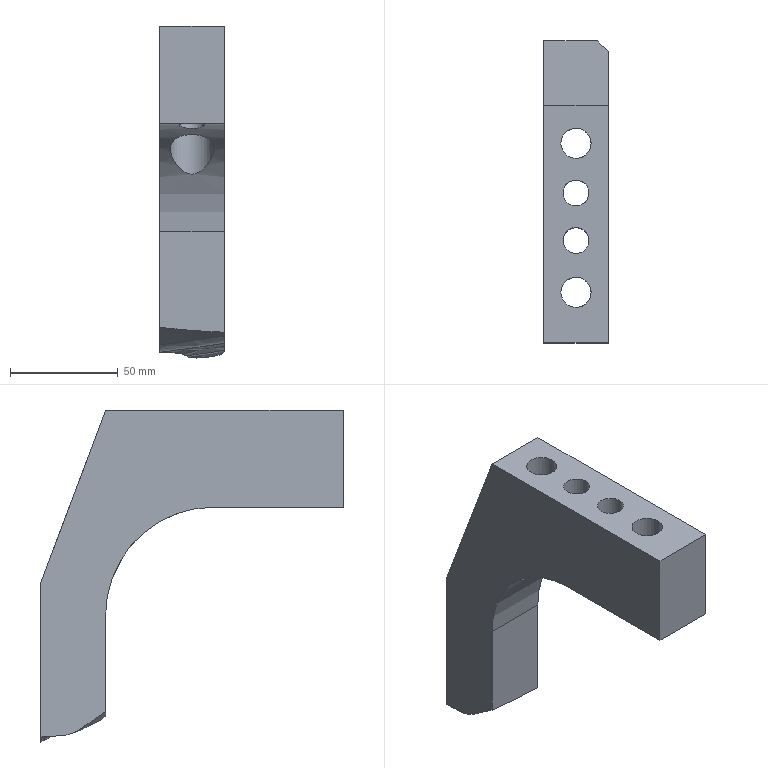Part | NX | features solid 2 | 1 solid | 24 faces | box 30.003 x 140.006 x 153.73 mm | volume 225991 mm3 | plane 11 | cylinder 7 | spline 6 | commonest cylinder face diameters 12 x2 14 x2 20 x2 100 x1
STEP:
#1=CARTESIAN_POINT('',(595.389,275.,-50.88));
#2=VERTEX_POINT('',#1);
#3=CARTESIAN_POINT('',(595.389,274.602,-50.209));
#4=VERTEX_POINT('',#3);
#5=CARTESIAN_POINT('',(595.389,275.,-50.88));
#6=CARTESIAN_POINT('',(595.389,274.842,-50.675));
#7=CARTESIAN_POINT('',(595.389,274.707,-50.449));
#8=CARTESIAN_POINT('',(595.389,274.602,-50.209));
#9=B_SPLINE_CURVE_WITH_KNOTS('',3,(#5,#6,#7,#8),.UNSPECIFIED.,.F.,.F.,(4,4),(0.002934,0.003708),.UNSPECIFIED.);
#10=EDGE_CURVE('',#2,#4,#9,.T.);
#11=ORIENTED_EDGE('',*,*,#10,.F.);
#12=CARTESIAN_POINT('',(595.389,275.,33.333));
#13=VERTEX_POINT('',#12);
#14=CARTESIAN_POINT('',(595.389,275.,20.));
#15=DIRECTION('',(0.,0.,1.));
#16=VECTOR('',#15,1000.);
#17=LINE('',#14,#16);
#18=EDGE_CURVE('',#2,#13,#17,.T.);
#19=ORIENTED_EDGE('',*,*,#18,.T.);
#20=CARTESIAN_POINT('',(595.389,250.,100.));
#21=VERTEX_POINT('',#20);
#22=CARTESIAN_POINT('',(595.389,339.439,-138.505));
#23=DIRECTION('',(0.,0.3511,-0.9363));
#24=VECTOR('',#23,1000.);
#25=LINE('',#22,#24);
#26=EDGE_CURVE('',#13,#21,#25,.F.);
#27=ORIENTED_EDGE('',*,*,#26,.T.);
#28=CARTESIAN_POINT('',(595.389,140.,100.));
#29=VERTEX_POINT('',#28);
#30=CARTESIAN_POINT('',(595.389,175.452,100.));
#31=DIRECTION('',(0.,1.,0.));
#32=VECTOR('',#31,1000.);
#33=LINE('',#30,#32);
#34=EDGE_CURVE('',#29,#21,#33,.T.);
#35=ORIENTED_EDGE('',*,*,#34,.F.);
#36=CARTESIAN_POINT('',(595.389,140.,55.));
#37=VERTEX_POINT('',#36);
#38=CARTESIAN_POINT('',(595.389,140.,-200.));
#39=DIRECTION('',(0.,0.,1.));
#40=VECTOR('',#39,1000.);
#41=LINE('',#38,#40);
#42=EDGE_CURVE('',#37,#29,#41,.T.);
#43=ORIENTED_EDGE('',*,*,#42,.F.);
#44=CARTESIAN_POINT('',(595.389,200.,55.));
#45=VERTEX_POINT('',#44);
#46=CARTESIAN_POINT('',(595.389,175.452,55.));
#47=DIRECTION('',(0.,1.,0.));
#48=VECTOR('',#47,1000.);
#49=LINE('',#46,#48);
#50=EDGE_CURVE('',#37,#45,#49,.T.);
#51=ORIENTED_EDGE('',*,*,#50,.T.);
#52=CARTESIAN_POINT('',(595.389,250.,5.));
#53=VERTEX_POINT('',#52);
#54=CARTESIAN_POINT('',(595.389,200.,5.));
#55=DIRECTION('',(1.,0.,0.));
#56=DIRECTION('',(0.,1.,0.));
#57=AXIS2_PLACEMENT_3D('',#54,#55,#56);
#58=CIRCLE('',#57,50.);
#59=EDGE_CURVE('',#45,#53,#58,.F.);
#60=ORIENTED_EDGE('',*,*,#59,.T.);
#61=CARTESIAN_POINT('',(595.389,250.,-41.794));
#62=VERTEX_POINT('',#61);
#63=CARTESIAN_POINT('',(595.389,250.,-200.));
#64=DIRECTION('',(0.,0.,1.));
#65=VECTOR('',#64,1000.);
#66=LINE('',#63,#65);
#67=EDGE_CURVE('',#62,#53,#66,.T.);
#68=ORIENTED_EDGE('',*,*,#67,.F.);
#69=CARTESIAN_POINT('',(595.389,252.457,-43.548));
#70=VERTEX_POINT('',#69);
#71=CARTESIAN_POINT('',(595.389,252.459,-43.549));
#72=CARTESIAN_POINT('',(595.389,251.639,-42.964));
#73=CARTESIAN_POINT('',(595.389,250.82,-42.379));
#74=CARTESIAN_POINT('',(595.389,250.,-41.794));
#75=B_SPLINE_CURVE_WITH_KNOTS('',3,(#71,#72,#73,#74),.UNSPECIFIED.,.F.,.F.,(4,4),(0.0001783,0.003199),.UNSPECIFIED.);
#76=EDGE_CURVE('',#70,#62,#75,.T.);
#77=ORIENTED_EDGE('',*,*,#76,.F.);
#78=CARTESIAN_POINT('',(595.389,262.065,-46.788));
#79=VERTEX_POINT('',#78);
#80=CARTESIAN_POINT('',(595.389,262.069,-46.789));
#81=CARTESIAN_POINT('',(595.389,258.623,-46.693));
#82=CARTESIAN_POINT('',(595.389,255.262,-45.551));
#83=CARTESIAN_POINT('',(595.389,252.457,-43.548));
#84=B_SPLINE_CURVE_WITH_KNOTS('',3,(#80,#81,#82,#83),.UNSPECIFIED.,.F.,.F.,(4,4),(0.,0.01023),.UNSPECIFIED.);
#85=EDGE_CURVE('',#79,#70,#84,.T.);
#86=ORIENTED_EDGE('',*,*,#85,.F.);
#87=CARTESIAN_POINT('',(595.389,269.735,-46.971));
#88=VERTEX_POINT('',#87);
#89=CARTESIAN_POINT('',(595.389,262.064,-46.788));
#90=CARTESIAN_POINT('',(595.389,264.616,-46.859));
#91=CARTESIAN_POINT('',(595.389,267.169,-46.92));
#92=CARTESIAN_POINT('',(595.389,269.721,-46.971));
#93=B_SPLINE_CURVE_WITH_KNOTS('',3,(#89,#90,#91,#92),.UNSPECIFIED.,.F.,.F.,(4,4),(0.0001094,0.007768),.UNSPECIFIED.);
#94=EDGE_CURVE('',#79,#88,#93,.T.);
#95=ORIENTED_EDGE('',*,*,#94,.T.);
#96=CARTESIAN_POINT('',(595.389,274.603,-50.211));
#97=CARTESIAN_POINT('',(595.389,273.774,-48.31));
#98=CARTESIAN_POINT('',(595.389,271.814,-47.013));
#99=CARTESIAN_POINT('',(595.389,269.74,-46.971));
#100=B_SPLINE_CURVE_WITH_KNOTS('',3,(#96,#97,#98,#99),.UNSPECIFIED.,.F.,.F.,(4,4),(0.,0.006132),.UNSPECIFIED.);
#101=EDGE_CURVE('',#4,#88,#100,.T.);
#102=ORIENTED_EDGE('',*,*,#101,.F.);
#103=EDGE_LOOP('',(#11,#19,#27,#35,#43,#51,#60,#68,#77,#86,#95,#102));
#104=FACE_BOUND('',#103,.T.);
#105=CARTESIAN_POINT('',(595.389,175.452,-200.));
#106=DIRECTION('',(1.,0.,0.));
#107=DIRECTION('',(0.,0.,-1.));
#108=AXIS2_PLACEMENT_3D('',#105,#106,#107);
#109=PLANE('',#108);
#110=ADVANCED_FACE('',(#104),#109,.T.);
#111=CARTESIAN_POINT('',(565.389,140.,100.));
#112=VERTEX_POINT('',#111);
#113=CARTESIAN_POINT('',(565.389,250.,100.));
#114=VERTEX_POINT('',#113);
#115=CARTESIAN_POINT('',(565.389,175.452,100.));
#116=DIRECTION('',(0.,1.,0.));
#117=VECTOR('',#116,1000.);
#118=LINE('',#115,#117);
#119=EDGE_CURVE('',#112,#114,#118,.T.);
#120=ORIENTED_EDGE('',*,*,#119,.T.);
#121=CARTESIAN_POINT('',(565.389,280.,20.));
#122=VERTEX_POINT('',#121);
#123=CARTESIAN_POINT('',(565.389,250.,100.));
#124=DIRECTION('',(0.,-0.3511,0.9363));
#125=VECTOR('',#124,1000.);
#126=LINE('',#123,#125);
#127=EDGE_CURVE('',#114,#122,#126,.F.);
#128=ORIENTED_EDGE('',*,*,#127,.T.);
#129=CARTESIAN_POINT('',(565.389,280.,-51.188));
#130=VERTEX_POINT('',#129);
#131=CARTESIAN_POINT('',(565.389,280.,-200.));
#132=DIRECTION('',(0.,0.,-1.));
#133=VECTOR('',#132,1000.);
#134=LINE('',#131,#133);
#135=EDGE_CURVE('',#122,#130,#134,.T.);
#136=ORIENTED_EDGE('',*,*,#135,.T.);
#137=CARTESIAN_POINT('',(565.389,279.203,-51.114));
#138=VERTEX_POINT('',#137);
#139=CARTESIAN_POINT('',(565.389,280.,-51.188));
#140=CARTESIAN_POINT('',(565.389,279.737,-51.145));
#141=CARTESIAN_POINT('',(565.389,279.473,-51.12));
#142=CARTESIAN_POINT('',(565.389,279.206,-51.114));
#143=B_SPLINE_CURVE_WITH_KNOTS('',3,(#139,#140,#141,#142),.UNSPECIFIED.,.F.,.F.,(4,4),(0.,0.0007971),.UNSPECIFIED.);
#144=EDGE_CURVE('',#130,#138,#143,.T.);
#145=ORIENTED_EDGE('',*,*,#144,.T.);
#146=CARTESIAN_POINT('',(565.389,271.356,-50.91));
#147=VERTEX_POINT('',#146);
#148=CARTESIAN_POINT('',(565.389,271.354,-50.91));
#149=CARTESIAN_POINT('',(565.389,273.966,-50.989));
#150=CARTESIAN_POINT('',(565.389,276.579,-51.057));
#151=CARTESIAN_POINT('',(565.389,279.191,-51.114));
#152=B_SPLINE_CURVE_WITH_KNOTS('',3,(#148,#149,#150,#151),.UNSPECIFIED.,.F.,.F.,(4,4),(0.00007643,0.007916),.UNSPECIFIED.);
#153=EDGE_CURVE('',#147,#138,#152,.T.);
#154=ORIENTED_EDGE('',*,*,#153,.F.);
#155=CARTESIAN_POINT('',(565.389,261.52,-47.642));
#156=VERTEX_POINT('',#155);
#157=CARTESIAN_POINT('',(565.389,271.357,-50.91));
#158=CARTESIAN_POINT('',(565.389,267.84,-50.803));
#159=CARTESIAN_POINT('',(565.389,264.401,-49.662));
#160=CARTESIAN_POINT('',(565.389,261.519,-47.641));
#161=B_SPLINE_CURVE_WITH_KNOTS('',3,(#157,#158,#159,#160),.UNSPECIFIED.,.F.,.F.,(4,4),(0.,0.01045),.UNSPECIFIED.);
#162=EDGE_CURVE('',#147,#156,#161,.T.);
#163=ORIENTED_EDGE('',*,*,#162,.T.);
#164=CARTESIAN_POINT('',(565.389,250.,-39.567));
#165=VERTEX_POINT('',#164);
#166=CARTESIAN_POINT('',(565.389,261.522,-47.643));
#167=CARTESIAN_POINT('',(565.389,257.681,-44.95));
#168=CARTESIAN_POINT('',(565.389,253.841,-42.258));
#169=CARTESIAN_POINT('',(565.389,250.,-39.567));
#170=B_SPLINE_CURVE_WITH_KNOTS('',3,(#166,#167,#168,#169),.UNSPECIFIED.,.F.,.F.,(4,4),(0.0001843,0.01425),.UNSPECIFIED.);
#171=EDGE_CURVE('',#156,#165,#170,.T.);
#172=ORIENTED_EDGE('',*,*,#171,.T.);
#173=CARTESIAN_POINT('',(565.389,250.,5.));
#174=VERTEX_POINT('',#173);
#175=CARTESIAN_POINT('',(565.389,250.,-200.));
#176=DIRECTION('',(0.,0.,1.));
#177=VECTOR('',#176,1000.);
#178=LINE('',#175,#177);
#179=EDGE_CURVE('',#165,#174,#178,.T.);
#180=ORIENTED_EDGE('',*,*,#179,.T.);
#181=CARTESIAN_POINT('',(565.389,200.,55.));
#182=VERTEX_POINT('',#181);
#183=CARTESIAN_POINT('',(565.389,200.,5.));
#184=DIRECTION('',(1.,0.,0.));
#185=DIRECTION('',(0.,1.,0.));
#186=AXIS2_PLACEMENT_3D('',#183,#184,#185);
#187=CIRCLE('',#186,50.);
#188=EDGE_CURVE('',#174,#182,#187,.T.);
#189=ORIENTED_EDGE('',*,*,#188,.T.);
#190=CARTESIAN_POINT('',(565.389,140.,55.));
#191=VERTEX_POINT('',#190);
#192=CARTESIAN_POINT('',(565.389,255.452,55.));
#193=DIRECTION('',(0.,1.,0.));
#194=VECTOR('',#193,1000.);
#195=LINE('',#192,#194);
#196=EDGE_CURVE('',#182,#191,#195,.F.);
#197=ORIENTED_EDGE('',*,*,#196,.T.);
#198=CARTESIAN_POINT('',(565.389,140.,-200.));
#199=DIRECTION('',(0.,0.,1.));
#200=VECTOR('',#199,1000.);
#201=LINE('',#198,#200);
#202=EDGE_CURVE('',#191,#112,#201,.T.);
#203=ORIENTED_EDGE('',*,*,#202,.T.);
#204=EDGE_LOOP('',(#120,#128,#136,#145,#154,#163,#172,#180,#189,#197,#203));
#205=FACE_BOUND('',#204,.T.);
#206=CARTESIAN_POINT('',(565.389,175.452,-200.));
#207=DIRECTION('',(1.,0.,0.));
#208=DIRECTION('',(0.,0.,-1.));
#209=AXIS2_PLACEMENT_3D('',#206,#207,#208);
#210=PLANE('',#209);
#211=ADVANCED_FACE('',(#205),#210,.F.);
#212=CARTESIAN_POINT('',(575.439,227.503,100.));
#213=VERTEX_POINT('',#212);
#214=CARTESIAN_POINT('',(580.389,232.452,100.));
#215=DIRECTION('',(0.,0.,-1.));
#216=DIRECTION('',(-0.7071,-0.7071,0.));
#217=AXIS2_PLACEMENT_3D('',#214,#215,#216);
#218=CIRCLE('',#217,7.);
#219=EDGE_CURVE('',#213,#213,#218,.T.);
#220=ORIENTED_EDGE('',*,*,#219,.T.);
#221=EDGE_LOOP('',(#220));
#222=FACE_BOUND('',#221,.T.);
#223=CARTESIAN_POINT('',(575.439,158.503,100.));
#224=VERTEX_POINT('',#223);
#225=CARTESIAN_POINT('',(580.389,163.452,100.));
#226=DIRECTION('',(0.,0.,-1.));
#227=DIRECTION('',(-0.7071,-0.7071,0.));
#228=AXIS2_PLACEMENT_3D('',#225,#226,#227);
#229=CIRCLE('',#228,7.);
#230=EDGE_CURVE('',#224,#224,#229,.T.);
#231=ORIENTED_EDGE('',*,*,#230,.T.);
#232=EDGE_LOOP('',(#231));
#233=FACE_BOUND('',#232,.T.);
#234=CARTESIAN_POINT('',(576.146,205.21,100.));
#235=VERTEX_POINT('',#234);
#236=CARTESIAN_POINT('',(580.389,209.452,100.));
#237=DIRECTION('',(0.,0.,-1.));
#238=DIRECTION('',(-0.7071,-0.7071,0.));
#239=AXIS2_PLACEMENT_3D('',#236,#237,#238);
#240=CIRCLE('',#239,6.);
#241=EDGE_CURVE('',#235,#235,#240,.T.);
#242=ORIENTED_EDGE('',*,*,#241,.T.);
#243=EDGE_LOOP('',(#242));
#244=FACE_BOUND('',#243,.T.);
#245=CARTESIAN_POINT('',(576.146,183.21,100.));
#246=VERTEX_POINT('',#245);
#247=CARTESIAN_POINT('',(580.389,187.452,100.));
#248=DIRECTION('',(0.,0.,-1.));
#249=DIRECTION('',(-0.7071,-0.7071,0.));
#250=AXIS2_PLACEMENT_3D('',#247,#248,#249);
#251=CIRCLE('',#250,6.);
#252=EDGE_CURVE('',#246,#246,#251,.T.);
#253=ORIENTED_EDGE('',*,*,#252,.T.);
#254=EDGE_LOOP('',(#253));
#255=FACE_BOUND('',#254,.T.);
#256=ORIENTED_EDGE('',*,*,#34,.T.);
#257=CARTESIAN_POINT('',(520.389,250.,100.));
#258=DIRECTION('',(-1.,0.,0.));
#259=VECTOR('',#258,1000.);
#260=LINE('',#257,#259);
#261=EDGE_CURVE('',#21,#114,#260,.T.);
#262=ORIENTED_EDGE('',*,*,#261,.T.);
#263=ORIENTED_EDGE('',*,*,#119,.F.);
#264=CARTESIAN_POINT('',(635.389,140.,100.));
#265=DIRECTION('',(-1.,0.,0.));
#266=VECTOR('',#265,1000.);
#267=LINE('',#264,#266);
#268=EDGE_CURVE('',#29,#112,#267,.T.);
#269=ORIENTED_EDGE('',*,*,#268,.F.);
#270=EDGE_LOOP('',(#256,#262,#263,#269));
#271=FACE_BOUND('',#270,.T.);
#272=CARTESIAN_POINT('',(520.389,175.452,100.));
#273=DIRECTION('',(0.,0.,-1.));
#274=DIRECTION('',(-1.,0.,0.));
#275=AXIS2_PLACEMENT_3D('',#272,#273,#274);
#276=PLANE('',#275);
#277=ADVANCED_FACE('',(#222,#233,#244,#255,#271),#276,.F.);
#278=CARTESIAN_POINT('',(590.389,163.452,55.));
#279=VERTEX_POINT('',#278);
#280=CARTESIAN_POINT('',(580.389,163.452,55.));
#281=DIRECTION('',(0.,0.,1.));
#282=DIRECTION('',(1.,0.,0.));
#283=AXIS2_PLACEMENT_3D('',#280,#281,#282);
#284=CIRCLE('',#283,10.);
#285=EDGE_CURVE('',#279,#279,#284,.F.);
#286=ORIENTED_EDGE('',*,*,#285,.F.);
#287=EDGE_LOOP('',(#286));
#288=FACE_BOUND('',#287,.T.);
#289=CARTESIAN_POINT('',(574.389,187.452,55.));
#290=VERTEX_POINT('',#289);
#291=CARTESIAN_POINT('',(580.389,187.452,55.));
#292=DIRECTION('',(0.,0.,-1.));
#293=DIRECTION('',(-1.,0.,0.));
#294=AXIS2_PLACEMENT_3D('',#291,#292,#293);
#295=CIRCLE('',#294,6.);
#296=EDGE_CURVE('',#290,#290,#295,.T.);
#297=ORIENTED_EDGE('',*,*,#296,.F.);
#298=EDGE_LOOP('',(#297));
#299=FACE_BOUND('',#298,.T.);
#300=ORIENTED_EDGE('',*,*,#196,.F.);
#301=CARTESIAN_POINT('',(595.389,200.,55.));
#302=DIRECTION('',(-1.,0.,0.));
#303=VECTOR('',#302,1000.);
#304=LINE('',#301,#303);
#305=EDGE_CURVE('',#182,#45,#304,.F.);
#306=ORIENTED_EDGE('',*,*,#305,.T.);
#307=ORIENTED_EDGE('',*,*,#50,.F.);
#308=CARTESIAN_POINT('',(595.389,140.,55.));
#309=DIRECTION('',(-1.,0.,0.));
#310=VECTOR('',#309,1000.);
#311=LINE('',#308,#310);
#312=EDGE_CURVE('',#37,#191,#311,.T.);
#313=ORIENTED_EDGE('',*,*,#312,.T.);
#314=EDGE_LOOP('',(#300,#306,#307,#313));
#315=FACE_BOUND('',#314,.T.);
#316=CARTESIAN_POINT('',(595.389,255.452,55.));
#317=DIRECTION('',(0.,0.,1.));
#318=DIRECTION('',(1.,0.,0.));
#319=AXIS2_PLACEMENT_3D('',#316,#317,#318);
#320=PLANE('',#319);
#321=ADVANCED_FACE('',(#288,#299,#315),#320,.F.);
#322=ORIENTED_EDGE('',*,*,#202,.F.);
#323=ORIENTED_EDGE('',*,*,#312,.F.);
#324=ORIENTED_EDGE('',*,*,#42,.T.);
#325=ORIENTED_EDGE('',*,*,#268,.T.);
#326=EDGE_LOOP('',(#322,#323,#324,#325));
#327=FACE_BOUND('',#326,.T.);
#328=CARTESIAN_POINT('',(635.389,140.,75.));
#329=DIRECTION('',(0.,1.,0.));
#330=DIRECTION('',(0.,0.,1.));
#331=AXIS2_PLACEMENT_3D('',#328,#329,#330);
#332=PLANE('',#331);
#333=ADVANCED_FACE('',(#327),#332,.F.);
#334=CARTESIAN_POINT('',(587.389,232.452,75.));
#335=VERTEX_POINT('',#334);
#336=CARTESIAN_POINT('',(580.389,232.452,75.));
#337=DIRECTION('',(0.,0.,1.));
#338=DIRECTION('',(1.,0.,0.));
#339=AXIS2_PLACEMENT_3D('',#336,#337,#338);
#340=CIRCLE('',#339,7.);
#341=EDGE_CURVE('',#335,#335,#340,.T.);
#342=ORIENTED_EDGE('',*,*,#341,.F.);
#343=EDGE_LOOP('',(#342));
#344=FACE_BOUND('',#343,.T.);
#345=ORIENTED_EDGE('',*,*,#219,.F.);
#346=EDGE_LOOP('',(#345));
#347=FACE_BOUND('',#346,.T.);
#348=CARTESIAN_POINT('',(580.389,232.452,75.));
#349=DIRECTION('',(0.,0.,1.));
#350=DIRECTION('',(-1.,0.,0.));
#351=AXIS2_PLACEMENT_3D('',#348,#349,#350);
#352=CYLINDRICAL_SURFACE('',#351,7.);
#353=ADVANCED_FACE('',(#344,#347),#352,.F.);
#354=ORIENTED_EDGE('',*,*,#341,.T.);
#355=EDGE_LOOP('',(#354));
#356=FACE_BOUND('',#355,.T.);
#357=CARTESIAN_POINT('',(590.389,232.452,75.));
#358=VERTEX_POINT('',#357);
#359=CARTESIAN_POINT('',(580.389,232.452,75.));
#360=DIRECTION('',(0.,0.,-1.));
#361=DIRECTION('',(1.,0.,0.));
#362=AXIS2_PLACEMENT_3D('',#359,#360,#361);
#363=CIRCLE('',#362,10.);
#364=EDGE_CURVE('',#358,#358,#363,.T.);
#365=ORIENTED_EDGE('',*,*,#364,.T.);
#366=EDGE_LOOP('',(#365));
#367=FACE_BOUND('',#366,.T.);
#368=CARTESIAN_POINT('',(580.389,232.452,75.));
#369=DIRECTION('',(0.,0.,1.));
#370=DIRECTION('',(-1.,0.,0.));
#371=AXIS2_PLACEMENT_3D('',#368,#369,#370);
#372=PLANE('',#371);
#373=ADVANCED_FACE('',(#356,#367),#372,.F.);
#374=CARTESIAN_POINT('',(571.633,227.622,46.677));
#375=VERTEX_POINT('',#374);
#376=CARTESIAN_POINT('',(574.156,224.201,48.791));
#377=CARTESIAN_POINT('',(571.35,227.566,46.791));
#378=CARTESIAN_POINT('',(570.238,231.271,44.109));
#379=CARTESIAN_POINT('',(570.471,234.796,41.005));
#380=CARTESIAN_POINT('',(571.78,237.887,37.725));
#381=CARTESIAN_POINT('',(573.658,240.016,35.024));
#382=CARTESIAN_POINT('',(575.727,241.369,33.098));
#383=CARTESIAN_POINT('',(577.614,242.141,31.917));
#384=CARTESIAN_POINT('',(579.896,242.535,31.281));
#385=CARTESIAN_POINT('',(582.271,242.362,31.564));
#386=CARTESIAN_POINT('',(584.326,241.718,32.574));
#387=CARTESIAN_POINT('',(586.565,240.483,34.386));
#388=CARTESIAN_POINT('',(588.607,238.463,37.042));
#389=CARTESIAN_POINT('',(590.116,235.478,40.331));
#390=CARTESIAN_POINT('',(590.592,232.039,43.482));
#391=CARTESIAN_POINT('',(589.784,228.323,46.286));
#392=CARTESIAN_POINT('',(587.347,224.824,48.449));
#393=CARTESIAN_POINT('',(583.305,222.502,49.656));
#394=CARTESIAN_POINT('',(578.48,222.255,49.774));
#395=CARTESIAN_POINT('',(574.156,224.201,48.791));
#396=CARTESIAN_POINT('',(571.35,227.566,46.791));
#397=CARTESIAN_POINT('',(570.238,231.271,44.109));
#398=B_SPLINE_CURVE_WITH_KNOTS('',3,(#376,#377,#378,#379,#380,#381,#382,#383,#384,#385,#386,#387,#388,#389,#390,#391,#392,#393,#394,#395,#396,#397),.UNSPECIFIED.,.T.,.F.,(1,1,1,1,1,1,1,1,1,1,1,1,1,1,1,1,1,1,1,1,1,1,1,1,1,1),(-0.01388,-0.009257,-0.004628,0.,0.004628,0.009257,0.01388,0.01851,0.02083,0.02314,0.02546,0.02777,0.03008,0.0324,0.03703,0.04165,0.04628,0.05091,0.05554,0.06017,0.0648,0.06942,0.07405,0.07868,0.08331,0.08794),.UNSPECIFIED.);
#399=EDGE_CURVE('',#375,#375,#398,.T.);
#400=ORIENTED_EDGE('',*,*,#399,.T.);
#401=EDGE_LOOP('',(#400));
#402=FACE_BOUND('',#401,.T.);
#403=ORIENTED_EDGE('',*,*,#364,.F.);
#404=EDGE_LOOP('',(#403));
#405=FACE_BOUND('',#404,.T.);
#406=CARTESIAN_POINT('',(580.389,232.452,75.));
#407=DIRECTION('',(0.,0.,-1.));
#408=DIRECTION('',(1.,0.,0.));
#409=AXIS2_PLACEMENT_3D('',#406,#407,#408);
#410=CYLINDRICAL_SURFACE('',#409,10.);
#411=ADVANCED_FACE('',(#402,#405),#410,.F.);
#412=CARTESIAN_POINT('',(587.389,163.452,75.));
#413=VERTEX_POINT('',#412);
#414=CARTESIAN_POINT('',(580.389,163.452,75.));
#415=DIRECTION('',(0.,0.,1.));
#416=DIRECTION('',(1.,0.,0.));
#417=AXIS2_PLACEMENT_3D('',#414,#415,#416);
#418=CIRCLE('',#417,7.);
#419=EDGE_CURVE('',#413,#413,#418,.T.);
#420=ORIENTED_EDGE('',*,*,#419,.F.);
#421=EDGE_LOOP('',(#420));
#422=FACE_BOUND('',#421,.T.);
#423=ORIENTED_EDGE('',*,*,#230,.F.);
#424=EDGE_LOOP('',(#423));
#425=FACE_BOUND('',#424,.T.);
#426=CARTESIAN_POINT('',(580.389,163.452,75.));
#427=DIRECTION('',(0.,0.,1.));
#428=DIRECTION('',(-1.,0.,0.));
#429=AXIS2_PLACEMENT_3D('',#426,#427,#428);
#430=CYLINDRICAL_SURFACE('',#429,7.);
#431=ADVANCED_FACE('',(#422,#425),#430,.F.);
#432=ORIENTED_EDGE('',*,*,#285,.T.);
#433=EDGE_LOOP('',(#432));
#434=FACE_BOUND('',#433,.T.);
#435=CARTESIAN_POINT('',(590.389,163.452,75.));
#436=VERTEX_POINT('',#435);
#437=CARTESIAN_POINT('',(580.389,163.452,75.));
#438=DIRECTION('',(0.,0.,-1.));
#439=DIRECTION('',(1.,0.,0.));
#440=AXIS2_PLACEMENT_3D('',#437,#438,#439);
#441=CIRCLE('',#440,10.);
#442=EDGE_CURVE('',#436,#436,#441,.T.);
#443=ORIENTED_EDGE('',*,*,#442,.F.);
#444=EDGE_LOOP('',(#443));
#445=FACE_BOUND('',#444,.T.);
#446=CARTESIAN_POINT('',(580.389,163.452,75.));
#447=DIRECTION('',(0.,0.,-1.));
#448=DIRECTION('',(1.,0.,0.));
#449=AXIS2_PLACEMENT_3D('',#446,#447,#448);
#450=CYLINDRICAL_SURFACE('',#449,10.);
#451=ADVANCED_FACE('',(#434,#445),#450,.F.);
#452=ORIENTED_EDGE('',*,*,#419,.T.);
#453=EDGE_LOOP('',(#452));
#454=FACE_BOUND('',#453,.T.);
#455=ORIENTED_EDGE('',*,*,#442,.T.);
#456=EDGE_LOOP('',(#455));
#457=FACE_BOUND('',#456,.T.);
#458=CARTESIAN_POINT('',(580.389,163.452,75.));
#459=DIRECTION('',(0.,0.,1.));
#460=DIRECTION('',(-1.,0.,0.));
#461=AXIS2_PLACEMENT_3D('',#458,#459,#460);
#462=PLANE('',#461);
#463=ADVANCED_FACE('',(#454,#457),#462,.F.);
#464=ORIENTED_EDGE('',*,*,#241,.F.);
#465=EDGE_LOOP('',(#464));
#466=FACE_BOUND('',#465,.T.);
#467=CARTESIAN_POINT('',(586.387,209.288,54.13));
#468=VERTEX_POINT('',#467);
#469=CARTESIAN_POINT('',(585.262,213.959,53.061));
#470=CARTESIAN_POINT('',(587.022,209.288,54.223));
#471=CARTESIAN_POINT('',(584.969,204.616,54.826));
#472=CARTESIAN_POINT('',(580.154,202.791,54.914));
#473=CARTESIAN_POINT('',(575.472,204.957,54.8));
#474=CARTESIAN_POINT('',(573.765,209.756,54.132));
#475=CARTESIAN_POINT('',(575.834,214.279,52.959));
#476=CARTESIAN_POINT('',(580.62,216.114,52.325));
#477=CARTESIAN_POINT('',(585.262,213.959,53.061));
#478=CARTESIAN_POINT('',(587.022,209.288,54.223));
#479=CARTESIAN_POINT('',(584.969,204.616,54.826));
#480=B_SPLINE_CURVE_WITH_KNOTS('',3,(#469,#470,#471,#472,#473,#474,#475,#476,#477,#478,#479),.UNSPECIFIED.,.T.,.F.,(1,1,1,1,1,1,1,1,1,1,1,1,1,1,1),(-0.01421,-0.009475,-0.004737,0.,0.004737,0.009475,0.01421,0.01895,0.02369,0.02842,0.03316,0.0379,0.04264,0.04737,0.05211),.UNSPECIFIED.);
#481=EDGE_CURVE('',#468,#468,#480,.T.);
#482=ORIENTED_EDGE('',*,*,#481,.T.);
#483=EDGE_LOOP('',(#482));
#484=FACE_BOUND('',#483,.T.);
#485=CARTESIAN_POINT('',(580.389,209.452,105.));
#486=DIRECTION('',(0.,0.,-1.));
#487=DIRECTION('',(-1.,0.,0.));
#488=AXIS2_PLACEMENT_3D('',#485,#486,#487);
#489=CYLINDRICAL_SURFACE('',#488,6.);
#490=ADVANCED_FACE('',(#466,#484),#489,.F.);
#491=ORIENTED_EDGE('',*,*,#252,.F.);
#492=EDGE_LOOP('',(#491));
#493=FACE_BOUND('',#492,.T.);
#494=ORIENTED_EDGE('',*,*,#296,.T.);
#495=EDGE_LOOP('',(#494));
#496=FACE_BOUND('',#495,.T.);
#497=CARTESIAN_POINT('',(580.389,187.452,105.));
#498=DIRECTION('',(0.,0.,-1.));
#499=DIRECTION('',(-1.,0.,0.));
#500=AXIS2_PLACEMENT_3D('',#497,#498,#499);
#501=CYLINDRICAL_SURFACE('',#500,6.);
#502=ADVANCED_FACE('',(#493,#496),#501,.F.);
#503=ORIENTED_EDGE('',*,*,#67,.T.);
#504=CARTESIAN_POINT('',(565.389,250.,5.));
#505=DIRECTION('',(-1.,0.,0.));
#506=VECTOR('',#505,1000.);
#507=LINE('',#504,#506);
#508=EDGE_CURVE('',#53,#174,#507,.T.);
#509=ORIENTED_EDGE('',*,*,#508,.T.);
#510=ORIENTED_EDGE('',*,*,#179,.F.);
#511=CARTESIAN_POINT('',(565.389,250.,-39.567));
#512=CARTESIAN_POINT('',(575.36,250.,-40.699));
#513=CARTESIAN_POINT('',(585.358,250.,-41.464));
#514=CARTESIAN_POINT('',(595.389,250.,-41.794));
#515=B_SPLINE_CURVE_WITH_KNOTS('',3,(#511,#512,#513,#514),.UNSPECIFIED.,.F.,.F.,(4,4),(0.,0.03008),.UNSPECIFIED.);
#516=EDGE_CURVE('',#165,#62,#515,.T.);
#517=ORIENTED_EDGE('',*,*,#516,.T.);
#518=EDGE_LOOP('',(#503,#509,#510,#517));
#519=FACE_BOUND('',#518,.T.);
#520=CARTESIAN_POINT('',(580.389,250.,4.472));
#521=DIRECTION('',(0.,1.,0.));
#522=DIRECTION('',(-1.,0.,0.));
#523=AXIS2_PLACEMENT_3D('',#520,#521,#522);
#524=PLANE('',#523);
#525=ADVANCED_FACE('',(#519),#524,.F.);
#526=CARTESIAN_POINT('',(590.389,280.,20.));
#527=VERTEX_POINT('',#526);
#528=CARTESIAN_POINT('',(580.389,280.,20.));
#529=DIRECTION('',(1.,0.,0.));
#530=VECTOR('',#529,1000.);
#531=LINE('',#528,#530);
#532=EDGE_CURVE('',#122,#527,#531,.T.);
#533=ORIENTED_EDGE('',*,*,#532,.T.);
#534=CARTESIAN_POINT('',(590.389,280.,-52.923));
#535=VERTEX_POINT('',#534);
#536=CARTESIAN_POINT('',(590.389,280.,-52.18));
#537=DIRECTION('',(0.,0.,-1.));
#538=VECTOR('',#537,1000.);
#539=LINE('',#536,#538);
#540=EDGE_CURVE('',#527,#535,#539,.T.);
#541=ORIENTED_EDGE('',*,*,#540,.T.);
#542=CARTESIAN_POINT('',(586.939,280.,-53.416));
#543=VERTEX_POINT('',#542);
#544=CARTESIAN_POINT('',(590.389,280.,-52.923));
#545=CARTESIAN_POINT('',(589.232,280.,-53.091));
#546=CARTESIAN_POINT('',(588.074,280.,-53.257));
#547=CARTESIAN_POINT('',(586.917,280.,-53.42));
#548=B_SPLINE_CURVE_WITH_KNOTS('',3,(#544,#545,#546,#547),.UNSPECIFIED.,.F.,.F.,(4,4),(0.005054,0.008561),.UNSPECIFIED.);
#549=EDGE_CURVE('',#535,#543,#548,.T.);
#550=ORIENTED_EDGE('',*,*,#549,.T.);
#551=CARTESIAN_POINT('',(577.508,280.,-52.788));
#552=VERTEX_POINT('',#551);
#553=CARTESIAN_POINT('',(586.96,280.,-53.413));
#554=CARTESIAN_POINT('',(585.374,280.,-53.637));
#555=CARTESIAN_POINT('',(582.969,280.,-53.826));
#556=CARTESIAN_POINT('',(579.782,280.,-53.577));
#557=CARTESIAN_POINT('',(578.2,280.,-53.206));
#558=CARTESIAN_POINT('',(577.509,280.,-52.788));
#559=B_SPLINE_CURVE_WITH_KNOTS('',3,(#553,#554,#555,#556,#557,#558),.UNSPECIFIED.,.F.,.F.,(4,1,1,4),(0.,0.004801,0.007201,0.009601),.UNSPECIFIED.);
#560=EDGE_CURVE('',#543,#552,#559,.T.);
#561=ORIENTED_EDGE('',*,*,#560,.T.);
#562=CARTESIAN_POINT('',(577.51,280.,-52.789));
#563=CARTESIAN_POINT('',(576.618,280.,-52.25));
#564=CARTESIAN_POINT('',(574.631,280.,-51.648));
#565=CARTESIAN_POINT('',(570.552,280.,-51.051));
#566=CARTESIAN_POINT('',(567.449,280.,-51.056));
#567=CARTESIAN_POINT('',(565.389,280.,-51.188));
#568=B_SPLINE_CURVE_WITH_KNOTS('',3,(#562,#563,#564,#565,#566,#567),.UNSPECIFIED.,.F.,.F.,(4,1,1,4),(0.,0.003084,0.006167,0.01233),.UNSPECIFIED.);
#569=EDGE_CURVE('',#552,#130,#568,.T.);
#570=ORIENTED_EDGE('',*,*,#569,.T.);
#571=ORIENTED_EDGE('',*,*,#135,.F.);
#572=EDGE_LOOP('',(#533,#541,#550,#561,#570,#571));
#573=FACE_BOUND('',#572,.T.);
#574=CARTESIAN_POINT('',(580.389,280.,77.5));
#575=DIRECTION('',(0.,-1.,0.));
#576=DIRECTION('',(1.,0.,0.));
#577=AXIS2_PLACEMENT_3D('',#574,#575,#576);
#578=PLANE('',#577);
#579=ADVANCED_FACE('',(#573),#578,.F.);
#580=ORIENTED_EDGE('',*,*,#85,.T.);
#581=CARTESIAN_POINT('',(595.388,252.457,-43.548));
#582=CARTESIAN_POINT('',(585.214,255.127,-45.11));
#583=CARTESIAN_POINT('',(575.214,258.15,-46.449));
#584=CARTESIAN_POINT('',(565.388,261.519,-47.641));
#585=B_SPLINE_CURVE_WITH_KNOTS('',3,(#581,#582,#583,#584),.UNSPECIFIED.,.F.,.F.,(4,4),(0.4564,0.6419),.UNSPECIFIED.);
#586=EDGE_CURVE('',#70,#156,#585,.T.);
#587=ORIENTED_EDGE('',*,*,#586,.T.);
#588=ORIENTED_EDGE('',*,*,#162,.F.);
#589=CARTESIAN_POINT('',(565.389,271.357,-50.91));
#590=CARTESIAN_POINT('',(575.205,267.905,-49.708));
#591=CARTESIAN_POINT('',(585.204,264.807,-48.361));
#592=CARTESIAN_POINT('',(595.389,262.069,-46.788));
#593=B_SPLINE_CURVE_WITH_KNOTS('',3,(#589,#590,#591,#592),.UNSPECIFIED.,.F.,.F.,(4,4),(0.3373,0.5274),.UNSPECIFIED.);
#594=EDGE_CURVE('',#147,#79,#593,.T.);
#595=ORIENTED_EDGE('',*,*,#594,.T.);
#596=EDGE_LOOP('',(#580,#587,#588,#595));
#597=FACE_BOUND('',#596,.T.);
#598=CARTESIAN_POINT('',(595.593,252.403,-43.516));
#599=CARTESIAN_POINT('',(596.178,253.928,-44.625));
#600=CARTESIAN_POINT('',(596.771,255.63,-45.486));
#601=CARTESIAN_POINT('',(597.354,257.461,-46.064));
#602=CARTESIAN_POINT('',(597.908,259.36,-46.34));
#603=CARTESIAN_POINT('',(598.416,261.267,-46.315));
#604=CARTESIAN_POINT('',(589.929,253.887,-44.387));
#605=CARTESIAN_POINT('',(590.527,255.405,-45.499));
#606=CARTESIAN_POINT('',(591.137,257.101,-46.362));
#607=CARTESIAN_POINT('',(591.741,258.925,-46.942));
#608=CARTESIAN_POINT('',(592.319,260.817,-47.219));
#609=CARTESIAN_POINT('',(592.853,262.718,-47.196));
#610=CARTESIAN_POINT('',(584.309,255.461,-45.201));
#611=CARTESIAN_POINT('',(584.92,256.974,-46.315));
#612=CARTESIAN_POINT('',(585.548,258.663,-47.18));
#613=CARTESIAN_POINT('',(586.173,260.479,-47.762));
#614=CARTESIAN_POINT('',(586.774,262.365,-48.041));
#615=CARTESIAN_POINT('',(587.335,264.259,-48.019));
#616=CARTESIAN_POINT('',(578.734,257.127,-45.963));
#617=CARTESIAN_POINT('',(579.359,258.633,-47.079));
#618=CARTESIAN_POINT('',(580.004,260.314,-47.947));
#619=CARTESIAN_POINT('',(580.651,262.123,-48.531));
#620=CARTESIAN_POINT('',(581.277,264.002,-48.811));
#621=CARTESIAN_POINT('',(581.863,265.888,-48.79));
#622=CARTESIAN_POINT('',(571.996,259.266,-46.835));
#623=CARTESIAN_POINT('',(572.639,260.763,-47.955));
#624=CARTESIAN_POINT('',(573.306,262.435,-48.825));
#625=CARTESIAN_POINT('',(573.978,264.235,-49.412));
#626=CARTESIAN_POINT('',(574.634,266.103,-49.694));
#627=CARTESIAN_POINT('',(575.252,267.981,-49.674));
#628=CARTESIAN_POINT('',(565.325,261.538,-47.65));
#629=CARTESIAN_POINT('',(565.985,263.026,-48.772));
#630=CARTESIAN_POINT('',(566.675,264.688,-49.645));
#631=CARTESIAN_POINT('',(567.373,266.478,-50.234));
#632=CARTESIAN_POINT('',(568.058,268.336,-50.518));
#633=CARTESIAN_POINT('',(568.707,270.203,-50.5));
#634=CARTESIAN_POINT('',(564.129,261.95,-47.795));
#635=CARTESIAN_POINT('',(564.793,263.437,-48.917));
#636=CARTESIAN_POINT('',(565.487,265.097,-49.791));
#637=CARTESIAN_POINT('',(566.19,266.885,-50.379));
#638=CARTESIAN_POINT('',(566.88,268.741,-50.664));
#639=CARTESIAN_POINT('',(567.535,270.606,-50.646));
#640=CARTESIAN_POINT('',(562.936,262.367,-47.937));
#641=CARTESIAN_POINT('',(563.603,263.851,-49.06));
#642=CARTESIAN_POINT('',(564.301,265.51,-49.934));
#643=CARTESIAN_POINT('',(565.009,267.296,-50.523));
#644=CARTESIAN_POINT('',(565.703,269.15,-50.809));
#645=CARTESIAN_POINT('',(566.364,271.014,-50.791));
#646=CARTESIAN_POINT('',(561.744,262.788,-48.078));
#647=CARTESIAN_POINT('',(562.414,264.271,-49.202));
#648=CARTESIAN_POINT('',(563.117,265.927,-50.076));
#649=CARTESIAN_POINT('',(563.829,267.711,-50.666));
#650=CARTESIAN_POINT('',(564.53,269.564,-50.951));
#651=CARTESIAN_POINT('',(565.196,271.425,-50.933));
#652=B_SPLINE_SURFACE_WITH_KNOTS('',5,5,((#598,#599,#600,#601,#602,#603),(#604,#605,#606,#607,#608,#609),(#610,#611,#612,#613,#614,#615),(#616,#617,#618,#619,#620,#621),(#622,#623,#624,#625,#626,#627),(#628,#629,#630,#631,#632,#633),(#634,#635,#636,#637,#638,#639),(#640,#641,#642,#643,#644,#645),(#646,#647,#648,#649,#650,#651)),.UNSPECIFIED.,.F.,.F.,.F.,(6,3,6),(6,6),(0.4552,0.6272,0.6648),(0.,1.),.UNSPECIFIED.);
#653=ADVANCED_FACE('',(#597),#652,.T.);
#654=ORIENTED_EDGE('',*,*,#594,.F.);
#655=ORIENTED_EDGE('',*,*,#153,.T.);
#656=CARTESIAN_POINT('',(565.386,279.192,-51.114));
#657=CARTESIAN_POINT('',(575.141,275.691,-49.913));
#658=CARTESIAN_POINT('',(585.138,272.528,-48.561));
#659=CARTESIAN_POINT('',(595.386,269.722,-46.971));
#660=B_SPLINE_CURVE_WITH_KNOTS('',3,(#656,#657,#658,#659),.UNSPECIFIED.,.F.,.F.,(4,4),(0.3631,0.5783),.UNSPECIFIED.);
#661=EDGE_CURVE('',#138,#88,#660,.T.);
#662=ORIENTED_EDGE('',*,*,#661,.T.);
#663=ORIENTED_EDGE('',*,*,#94,.F.);
#664=EDGE_LOOP('',(#654,#655,#662,#663));
#665=FACE_BOUND('',#664,.T.);
#666=CARTESIAN_POINT('',(595.57,261.935,-46.758));
#667=CARTESIAN_POINT('',(596.003,263.763,-46.745));
#668=CARTESIAN_POINT('',(596.436,265.591,-46.726));
#669=CARTESIAN_POINT('',(596.869,267.419,-46.702));
#670=CARTESIAN_POINT('',(597.302,269.247,-46.673));
#671=CARTESIAN_POINT('',(594.342,262.266,-46.948));
#672=CARTESIAN_POINT('',(594.781,264.092,-46.935));
#673=CARTESIAN_POINT('',(595.219,265.919,-46.916));
#674=CARTESIAN_POINT('',(595.658,267.745,-46.892));
#675=CARTESIAN_POINT('',(596.096,269.572,-46.863));
#676=CARTESIAN_POINT('',(593.116,262.601,-47.135));
#677=CARTESIAN_POINT('',(593.561,264.426,-47.122));
#678=CARTESIAN_POINT('',(594.005,266.251,-47.104));
#679=CARTESIAN_POINT('',(594.449,268.076,-47.079));
#680=CARTESIAN_POINT('',(594.893,269.901,-47.05));
#681=CARTESIAN_POINT('',(591.894,262.94,-47.319));
#682=CARTESIAN_POINT('',(592.344,264.763,-47.306));
#683=CARTESIAN_POINT('',(592.794,266.587,-47.288));
#684=CARTESIAN_POINT('',(593.244,268.41,-47.264));
#685=CARTESIAN_POINT('',(593.693,270.234,-47.234));
#686=CARTESIAN_POINT('',(585.233,264.816,-48.311));
#687=CARTESIAN_POINT('',(585.714,266.631,-48.299));
#688=CARTESIAN_POINT('',(586.194,268.446,-48.281));
#689=CARTESIAN_POINT('',(586.674,270.261,-48.257));
#690=CARTESIAN_POINT('',(587.154,272.076,-48.227));
#691=CARTESIAN_POINT('',(578.659,266.815,-49.225));
#692=CARTESIAN_POINT('',(579.17,268.621,-49.213));
#693=CARTESIAN_POINT('',(579.681,270.427,-49.196));
#694=CARTESIAN_POINT('',(580.191,272.233,-49.172));
#695=CARTESIAN_POINT('',(580.701,274.039,-49.143));
#696=CARTESIAN_POINT('',(573.347,268.53,-49.925));
#697=CARTESIAN_POINT('',(573.882,270.328,-49.914));
#698=CARTESIAN_POINT('',(574.417,272.126,-49.898));
#699=CARTESIAN_POINT('',(574.951,273.924,-49.875));
#700=CARTESIAN_POINT('',(575.485,275.722,-49.845));
#701=CARTESIAN_POINT('',(568.091,270.325,-50.586));
#702=CARTESIAN_POINT('',(568.65,272.114,-50.576));
#703=CARTESIAN_POINT('',(569.209,273.904,-50.559));
#704=CARTESIAN_POINT('',(569.768,275.694,-50.537));
#705=CARTESIAN_POINT('',(570.326,277.484,-50.508));
#706=CARTESIAN_POINT('',(562.892,272.198,-51.211));
#707=CARTESIAN_POINT('',(563.475,273.979,-51.202));
#708=CARTESIAN_POINT('',(564.058,275.761,-51.186));
#709=CARTESIAN_POINT('',(564.64,277.542,-51.164));
#710=CARTESIAN_POINT('',(565.222,279.323,-51.136));
#711=B_SPLINE_SURFACE_WITH_KNOTS('',5,4,((#666,#667,#668,#669,#670),(#671,#672,#673,#674,#675),(#676,#677,#678,#679,#680),(#681,#682,#683,#684,#685),(#686,#687,#688,#689,#690),(#691,#692,#693,#694,#695),(#696,#697,#698,#699,#700),(#701,#702,#703,#704,#705),(#706,#707,#708,#709,#710)),.UNSPECIFIED.,.F.,.F.,.F.,(6,3,6),(5,5),(0.4617,0.5,0.6709),(0.003646,0.9938),.UNSPECIFIED.);
#712=ADVANCED_FACE('',(#665),#711,.T.);
#713=ORIENTED_EDGE('',*,*,#101,.T.);
#714=ORIENTED_EDGE('',*,*,#661,.F.);
#715=ORIENTED_EDGE('',*,*,#144,.F.);
#716=ORIENTED_EDGE('',*,*,#569,.F.);
#717=CARTESIAN_POINT('',(595.389,274.602,-50.208));
#718=CARTESIAN_POINT('',(589.366,276.27,-51.14));
#719=CARTESIAN_POINT('',(583.404,278.07,-51.995));
#720=CARTESIAN_POINT('',(577.508,280.,-52.787));
#721=B_SPLINE_CURVE_WITH_KNOTS('',3,(#717,#718,#719,#720),.UNSPECIFIED.,.F.,.F.,(4,4),(0.4427,0.5704),.UNSPECIFIED.);
#722=EDGE_CURVE('',#4,#552,#721,.T.);
#723=ORIENTED_EDGE('',*,*,#722,.F.);
#724=EDGE_LOOP('',(#713,#714,#715,#716,#723));
#725=FACE_BOUND('',#724,.T.);
#726=CARTESIAN_POINT('',(597.234,274.097,-49.924));
#727=CARTESIAN_POINT('',(596.956,273.686,-48.85));
#728=CARTESIAN_POINT('',(596.614,272.96,-47.914));
#729=CARTESIAN_POINT('',(596.24,271.966,-47.242));
#730=CARTESIAN_POINT('',(595.882,270.831,-46.919));
#731=CARTESIAN_POINT('',(595.576,269.689,-46.942));
#732=CARTESIAN_POINT('',(593.682,275.063,-50.482));
#733=CARTESIAN_POINT('',(593.405,274.653,-49.408));
#734=CARTESIAN_POINT('',(593.06,273.929,-48.471));
#735=CARTESIAN_POINT('',(592.68,272.938,-47.798));
#736=CARTESIAN_POINT('',(592.314,271.806,-47.475));
#737=CARTESIAN_POINT('',(591.997,270.667,-47.498));
#738=CARTESIAN_POINT('',(590.147,276.067,-51.017));
#739=CARTESIAN_POINT('',(589.871,275.658,-49.942));
#740=CARTESIAN_POINT('',(589.524,274.937,-49.005));
#741=CARTESIAN_POINT('',(589.138,273.948,-48.331));
#742=CARTESIAN_POINT('',(588.762,272.819,-48.008));
#743=CARTESIAN_POINT('',(588.436,271.683,-48.031));
#744=CARTESIAN_POINT('',(586.629,277.109,-51.53));
#745=CARTESIAN_POINT('',(586.354,276.702,-50.455));
#746=CARTESIAN_POINT('',(586.004,275.982,-49.517));
#747=CARTESIAN_POINT('',(585.612,274.997,-48.843));
#748=CARTESIAN_POINT('',(585.228,273.871,-48.52));
#749=CARTESIAN_POINT('',(584.891,272.738,-48.543));
#750=CARTESIAN_POINT('',(580.537,278.989,-52.39));
#751=CARTESIAN_POINT('',(580.262,278.585,-51.314));
#752=CARTESIAN_POINT('',(579.908,277.869,-50.375));
#753=CARTESIAN_POINT('',(579.504,276.889,-49.701));
#754=CARTESIAN_POINT('',(579.105,275.769,-49.377));
#755=CARTESIAN_POINT('',(578.75,274.641,-49.399));
#756=CARTESIAN_POINT('',(574.502,280.983,-53.194));
#757=CARTESIAN_POINT('',(574.227,280.581,-52.117));
#758=CARTESIAN_POINT('',(573.867,279.87,-51.178));
#759=CARTESIAN_POINT('',(573.453,278.895,-50.502));
#760=CARTESIAN_POINT('',(573.037,277.781,-50.178));
#761=CARTESIAN_POINT('',(572.664,276.66,-50.2));
#762=CARTESIAN_POINT('',(571.943,281.853,-53.527));
#763=CARTESIAN_POINT('',(571.669,281.452,-52.449));
#764=CARTESIAN_POINT('',(571.306,280.742,-51.51));
#765=CARTESIAN_POINT('',(570.887,279.77,-50.834));
#766=CARTESIAN_POINT('',(570.464,278.659,-50.509));
#767=CARTESIAN_POINT('',(570.084,277.54,-50.531));
#768=CARTESIAN_POINT('',(569.396,282.743,-53.85));
#769=CARTESIAN_POINT('',(569.121,282.343,-52.773));
#770=CARTESIAN_POINT('',(568.755,281.635,-51.833));
#771=CARTESIAN_POINT('',(568.331,280.665,-51.157));
#772=CARTESIAN_POINT('',(567.902,279.557,-50.832));
#773=CARTESIAN_POINT('',(567.514,278.441,-50.853));
#774=CARTESIAN_POINT('',(566.859,283.653,-54.166));
#775=CARTESIAN_POINT('',(566.584,283.254,-53.088));
#776=CARTESIAN_POINT('',(566.216,282.548,-52.148));
#777=CARTESIAN_POINT('',(565.786,281.581,-51.472));
#778=CARTESIAN_POINT('',(565.35,280.475,-51.146));
#779=CARTESIAN_POINT('',(564.954,279.362,-51.168));
#780=B_SPLINE_SURFACE_WITH_KNOTS('',5,5,((#726,#727,#728,#729,#730,#731),(#732,#733,#734,#735,#736,#737),(#738,#739,#740,#741,#742,#743),(#744,#745,#746,#747,#748,#749),(#750,#751,#752,#753,#754,#755),(#756,#757,#758,#759,#760,#761),(#762,#763,#764,#765,#766,#767),(#768,#769,#770,#771,#772,#773),(#774,#775,#776,#777,#778,#779)),.UNSPECIFIED.,.F.,.F.,.F.,(6,3,6),(6,6),(0.4297,0.5549,0.6478),(0.,1.),.UNSPECIFIED.);
#781=ADVANCED_FACE('',(#725),#780,.F.);
#782=CARTESIAN_POINT('',(591.849,278.547,-52.693));
#783=VERTEX_POINT('',#782);
#784=CARTESIAN_POINT('',(591.851,278.553,-52.693));
#785=CARTESIAN_POINT('',(590.209,279.028,-52.94));
#786=CARTESIAN_POINT('',(588.572,279.512,-53.181));
#787=CARTESIAN_POINT('',(586.94,280.006,-53.416));
#788=B_SPLINE_CURVE_WITH_KNOTS('',3,(#784,#785,#786,#787),.UNSPECIFIED.,.F.,.F.,(4,4),(0.4721,0.5073),.UNSPECIFIED.);
#789=EDGE_CURVE('',#783,#543,#788,.T.);
#790=ORIENTED_EDGE('',*,*,#789,.F.);
#791=CARTESIAN_POINT('',(591.848,278.541,-52.693));
#792=CARTESIAN_POINT('',(593.112,277.277,-52.488));
#793=CARTESIAN_POINT('',(594.378,276.011,-51.982));
#794=CARTESIAN_POINT('',(595.389,275.,-50.88));
#795=B_SPLINE_CURVE_WITH_KNOTS('',3,(#791,#792,#793,#794),.UNSPECIFIED.,.F.,.F.,(4,4),(0.,0.005381),.UNSPECIFIED.);
#796=EDGE_CURVE('',#783,#2,#795,.T.);
#797=ORIENTED_EDGE('',*,*,#796,.T.);
#798=ORIENTED_EDGE('',*,*,#10,.T.);
#799=ORIENTED_EDGE('',*,*,#722,.T.);
#800=ORIENTED_EDGE('',*,*,#560,.F.);
#801=EDGE_LOOP('',(#790,#797,#798,#799,#800));
#802=FACE_BOUND('',#801,.T.);
#803=CARTESIAN_POINT('',(596.515,277.236,-51.979));
#804=CARTESIAN_POINT('',(596.327,276.547,-51.999));
#805=CARTESIAN_POINT('',(596.107,275.861,-51.809));
#806=CARTESIAN_POINT('',(595.877,275.259,-51.406));
#807=CARTESIAN_POINT('',(595.667,274.82,-50.841));
#808=CARTESIAN_POINT('',(595.497,274.572,-50.192));
#809=CARTESIAN_POINT('',(592.868,278.243,-52.548));
#810=CARTESIAN_POINT('',(592.674,277.555,-52.568));
#811=CARTESIAN_POINT('',(592.448,276.871,-52.378));
#812=CARTESIAN_POINT('',(592.215,276.27,-51.974));
#813=CARTESIAN_POINT('',(592.003,275.832,-51.409));
#814=CARTESIAN_POINT('',(591.834,275.586,-50.76));
#815=CARTESIAN_POINT('',(589.244,279.289,-53.092));
#816=CARTESIAN_POINT('',(589.043,278.603,-53.112));
#817=CARTESIAN_POINT('',(588.812,277.92,-52.922));
#818=CARTESIAN_POINT('',(588.574,277.322,-52.518));
#819=CARTESIAN_POINT('',(588.361,276.885,-51.952));
#820=CARTESIAN_POINT('',(588.193,276.639,-51.303));
#821=CARTESIAN_POINT('',(585.642,280.374,-53.614));
#822=CARTESIAN_POINT('',(585.434,279.69,-53.634));
#823=CARTESIAN_POINT('',(585.198,279.009,-53.444));
#824=CARTESIAN_POINT('',(584.956,278.412,-53.039));
#825=CARTESIAN_POINT('',(584.742,277.977,-52.473));
#826=CARTESIAN_POINT('',(584.573,277.732,-51.823));
#827=CARTESIAN_POINT('',(582.063,281.498,-54.114));
#828=CARTESIAN_POINT('',(581.849,280.816,-54.135));
#829=CARTESIAN_POINT('',(581.607,280.137,-53.944));
#830=CARTESIAN_POINT('',(581.361,279.542,-53.539));
#831=CARTESIAN_POINT('',(581.145,279.108,-52.973));
#832=CARTESIAN_POINT('',(580.976,278.864,-52.322));
#833=CARTESIAN_POINT('',(578.506,282.661,-54.596));
#834=CARTESIAN_POINT('',(578.286,281.981,-54.616));
#835=CARTESIAN_POINT('',(578.038,281.304,-54.425));
#836=CARTESIAN_POINT('',(577.789,280.711,-54.02));
#837=CARTESIAN_POINT('',(577.57,280.278,-53.453));
#838=CARTESIAN_POINT('',(577.402,280.035,-52.802));
#839=B_SPLINE_SURFACE_WITH_KNOTS('',5,5,((#803,#804,#805,#806,#807,#808),(#809,#810,#811,#812,#813,#814),(#815,#816,#817,#818,#819,#820),(#821,#822,#823,#824,#825,#826),(#827,#828,#829,#830,#831,#832),(#833,#834,#835,#836,#837,#838)),.UNSPECIFIED.,.F.,.F.,.F.,(6,6),(6,6),(0.4389,0.5683),(0.,1.),.PIECEWISE_BEZIER_KNOTS.);
#840=ADVANCED_FACE('',(#802),#839,.F.);
#841=ORIENTED_EDGE('',*,*,#549,.F.);
#842=CARTESIAN_POINT('',(590.389,280.,-52.923));
#843=CARTESIAN_POINT('',(590.875,279.514,-52.847));
#844=CARTESIAN_POINT('',(591.361,279.027,-52.77));
#845=CARTESIAN_POINT('',(591.848,278.541,-52.693));
#846=B_SPLINE_CURVE_WITH_KNOTS('',3,(#842,#843,#844,#845),.UNSPECIFIED.,.F.,.F.,(4,4),(0.,0.002076),.UNSPECIFIED.);
#847=EDGE_CURVE('',#535,#783,#846,.T.);
#848=ORIENTED_EDGE('',*,*,#847,.T.);
#849=ORIENTED_EDGE('',*,*,#789,.T.);
#850=EDGE_LOOP('',(#841,#848,#849));
#851=FACE_BOUND('',#850,.T.);
#852=CARTESIAN_POINT('',(591.875,278.525,-52.689));
#853=CARTESIAN_POINT('',(591.926,278.719,-52.684));
#854=CARTESIAN_POINT('',(591.977,278.914,-52.679));
#855=CARTESIAN_POINT('',(592.027,279.109,-52.674));
#856=CARTESIAN_POINT('',(592.078,279.304,-52.668));
#857=CARTESIAN_POINT('',(592.128,279.499,-52.663));
#858=CARTESIAN_POINT('',(590.873,278.815,-52.839));
#859=CARTESIAN_POINT('',(590.924,279.009,-52.834));
#860=CARTESIAN_POINT('',(590.975,279.204,-52.829));
#861=CARTESIAN_POINT('',(591.026,279.399,-52.824));
#862=CARTESIAN_POINT('',(591.078,279.593,-52.819));
#863=CARTESIAN_POINT('',(591.129,279.788,-52.814));
#864=CARTESIAN_POINT('',(589.873,279.107,-52.988));
#865=CARTESIAN_POINT('',(589.925,279.302,-52.983));
#866=CARTESIAN_POINT('',(589.976,279.496,-52.978));
#867=CARTESIAN_POINT('',(590.028,279.691,-52.973));
#868=CARTESIAN_POINT('',(590.08,279.885,-52.968));
#869=CARTESIAN_POINT('',(590.131,280.08,-52.962));
#870=CARTESIAN_POINT('',(588.875,279.403,-53.135));
#871=CARTESIAN_POINT('',(588.927,279.597,-53.13));
#872=CARTESIAN_POINT('',(588.979,279.792,-53.125));
#873=CARTESIAN_POINT('',(589.032,279.986,-53.12));
#874=CARTESIAN_POINT('',(589.084,280.181,-53.115));
#875=CARTESIAN_POINT('',(589.136,280.375,-53.109));
#876=CARTESIAN_POINT('',(587.879,279.702,-53.28));
#877=CARTESIAN_POINT('',(587.932,279.896,-53.275));
#878=CARTESIAN_POINT('',(587.985,280.09,-53.27));
#879=CARTESIAN_POINT('',(588.037,280.284,-53.265));
#880=CARTESIAN_POINT('',(588.09,280.479,-53.26));
#881=CARTESIAN_POINT('',(588.142,280.673,-53.255));
#882=CARTESIAN_POINT('',(586.886,280.003,-53.424));
#883=CARTESIAN_POINT('',(586.939,280.197,-53.419));
#884=CARTESIAN_POINT('',(586.992,280.391,-53.414));
#885=CARTESIAN_POINT('',(587.045,280.585,-53.409));
#886=CARTESIAN_POINT('',(587.098,280.78,-53.403));
#887=CARTESIAN_POINT('',(587.151,280.974,-53.398));
#888=B_SPLINE_SURFACE_WITH_KNOTS('',5,5,((#852,#853,#854,#855,#856,#857),(#858,#859,#860,#861,#862,#863),(#864,#865,#866,#867,#868,#869),(#870,#871,#872,#873,#874,#875),(#876,#877,#878,#879,#880,#881),(#882,#883,#884,#885,#886,#887)),.UNSPECIFIED.,.F.,.F.,.F.,(6,6),(6,6),(0.5587,0.5883),(0.6646,0.6957),.PIECEWISE_BEZIER_KNOTS.);
#889=ADVANCED_FACE('',(#851),#888,.T.);
#890=ORIENTED_EDGE('',*,*,#76,.T.);
#891=ORIENTED_EDGE('',*,*,#516,.F.);
#892=ORIENTED_EDGE('',*,*,#171,.F.);
#893=ORIENTED_EDGE('',*,*,#586,.F.);
#894=EDGE_LOOP('',(#890,#891,#892,#893));
#895=FACE_BOUND('',#894,.T.);
#896=CARTESIAN_POINT('',(596.434,252.254,-43.436));
#897=CARTESIAN_POINT('',(592.55,241.823,-35.864));
#898=CARTESIAN_POINT('',(590.116,253.896,-44.415));
#899=CARTESIAN_POINT('',(586.134,243.513,-36.826));
#900=CARTESIAN_POINT('',(583.833,255.656,-45.325));
#901=CARTESIAN_POINT('',(579.749,245.325,-37.719));
#902=CARTESIAN_POINT('',(577.592,257.535,-46.172));
#903=CARTESIAN_POINT('',(573.401,247.258,-38.55));
#904=CARTESIAN_POINT('',(571.394,259.531,-46.965));
#905=CARTESIAN_POINT('',(567.092,249.312,-39.328));
#906=CARTESIAN_POINT('',(565.233,261.647,-47.713));
#907=CARTESIAN_POINT('',(560.815,251.489,-40.062));
#908=B_SPLINE_SURFACE_WITH_KNOTS('',5,1,((#896,#897),(#898,#899),(#900,#901),(#902,#903),(#904,#905),(#906,#907)),.RULED_SURF.,.F.,.F.,.F.,(6,6),(2,2),(0.4618,0.6521),(0.003321,0.4958),.PIECEWISE_BEZIER_KNOTS.);
#909=ADVANCED_FACE('',(#895),#908,.F.);
#910=ORIENTED_EDGE('',*,*,#59,.F.);
#911=ORIENTED_EDGE('',*,*,#305,.F.);
#912=ORIENTED_EDGE('',*,*,#188,.F.);
#913=ORIENTED_EDGE('',*,*,#508,.F.);
#914=EDGE_LOOP('',(#910,#911,#912,#913));
#915=FACE_BOUND('',#914,.T.);
#916=ORIENTED_EDGE('',*,*,#481,.F.);
#917=EDGE_LOOP('',(#916));
#918=FACE_BOUND('',#917,.T.);
#919=ORIENTED_EDGE('',*,*,#399,.F.);
#920=EDGE_LOOP('',(#919));
#921=FACE_BOUND('',#920,.T.);
#922=CARTESIAN_POINT('',(580.389,200.,5.));
#923=DIRECTION('',(1.,0.,0.));
#924=DIRECTION('',(0.,1.,0.));
#925=AXIS2_PLACEMENT_3D('',#922,#923,#924);
#926=CYLINDRICAL_SURFACE('',#925,50.);
#927=ADVANCED_FACE('',(#915,#918,#921),#926,.F.);
#928=ORIENTED_EDGE('',*,*,#26,.F.);
#929=CARTESIAN_POINT('',(609.413,260.976,70.732));
#930=DIRECTION('',(0.3313,-0.3313,0.8835));
#931=VECTOR('',#930,1000.);
#932=LINE('',#929,#931);
#933=EDGE_CURVE('',#13,#527,#932,.F.);
#934=ORIENTED_EDGE('',*,*,#933,.T.);
#935=ORIENTED_EDGE('',*,*,#532,.F.);
#936=ORIENTED_EDGE('',*,*,#127,.F.);
#937=ORIENTED_EDGE('',*,*,#261,.F.);
#938=EDGE_LOOP('',(#928,#934,#935,#936,#937));
#939=FACE_BOUND('',#938,.T.);
#940=CARTESIAN_POINT('',(520.389,250.,100.));
#941=DIRECTION('',(0.,-0.9363,-0.3511));
#942=DIRECTION('',(0.,0.3511,-0.9363));
#943=AXIS2_PLACEMENT_3D('',#940,#941,#942);
#944=PLANE('',#943);
#945=ADVANCED_FACE('',(#939),#944,.F.);
#946=ORIENTED_EDGE('',*,*,#933,.F.);
#947=ORIENTED_EDGE('',*,*,#18,.F.);
#948=ORIENTED_EDGE('',*,*,#796,.F.);
#949=ORIENTED_EDGE('',*,*,#847,.F.);
#950=ORIENTED_EDGE('',*,*,#540,.F.);
#951=EDGE_LOOP('',(#946,#947,#948,#949,#950));
#952=FACE_BOUND('',#951,.T.);
#953=CARTESIAN_POINT('',(590.389,280.,77.5));
#954=DIRECTION('',(0.7071,0.7071,0.));
#955=DIRECTION('',(-0.7071,0.7071,0.));
#956=AXIS2_PLACEMENT_3D('',#953,#954,#955);
#957=PLANE('',#956);
#958=ADVANCED_FACE('',(#952),#957,.T.);
#959=CLOSED_SHELL('',(#110,#211,#277,#321,#333,#353,#373,#411,#431,#451,#463,#490,#502,#525,#579,#653,#712,#781,#840,#889,#909,#927,#945,#958));
#960=MANIFOLD_SOLID_BREP('',#959);
#961=(LENGTH_UNIT()NAMED_UNIT(*)SI_UNIT(.MILLI.,.METRE.));
#962=UNCERTAINTY_MEASURE_WITH_UNIT(LENGTH_MEASURE(0.1242),#961,'','');
#963=(NAMED_UNIT(*)PLANE_ANGLE_UNIT()SI_UNIT($,.RADIAN.));
#964=(NAMED_UNIT(*)SI_UNIT($,.STERADIAN.)SOLID_ANGLE_UNIT());
#965=(GEOMETRIC_REPRESENTATION_CONTEXT(3)GLOBAL_UNCERTAINTY_ASSIGNED_CONTEXT((#962))GLOBAL_UNIT_ASSIGNED_CONTEXT((#961,#963,#964))REPRESENTATION_CONTEXT('',''));
#966=ADVANCED_BREP_SHAPE_REPRESENTATION('',(#960),#965);